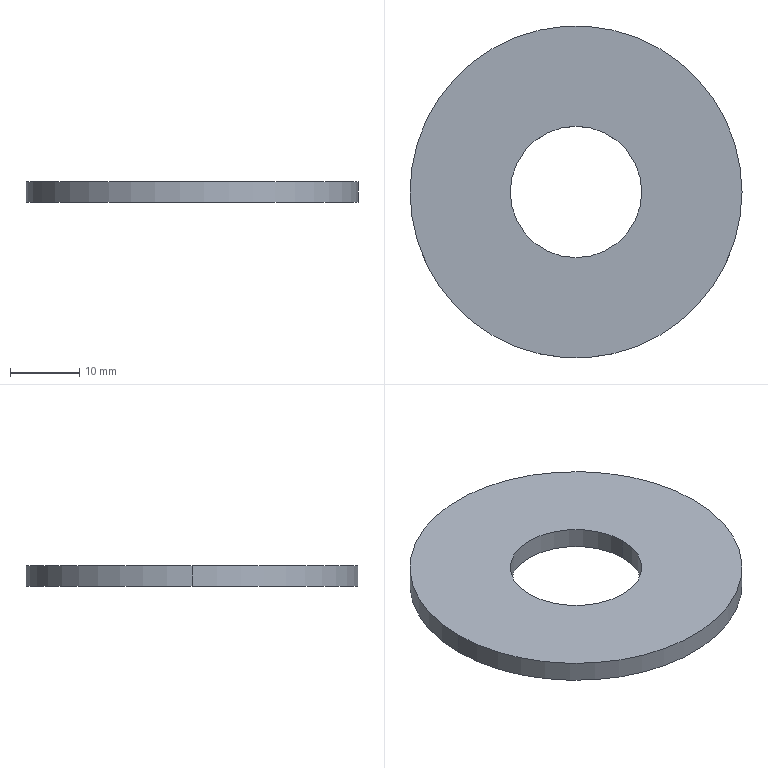Part | SolidWorks | features Extrusion 1 | 1 solid | 6 faces | box 48 x 48 x 3 mm | volume 4578 mm3 | cylinder 4 | plane 2 | commonest cylinder face diameters 19 x2 48 x2
STEP:
#1=CARTESIAN_POINT('',(-9.5,0.,3.));
#2=VERTEX_POINT('',#1);
#3=CARTESIAN_POINT('',(9.5,0.,3.));
#4=VERTEX_POINT('',#3);
#5=CARTESIAN_POINT('',(0.,0.,3.));
#6=DIRECTION('',(0.,0.,1.));
#7=DIRECTION('',(1.,0.,0.));
#8=AXIS2_PLACEMENT_3D('',#5,#6,#7);
#9=CIRCLE('',#8,9.5);
#10=EDGE_CURVE('',#2,#4,#9,.T.);
#11=ORIENTED_EDGE('',*,*,#10,.T.);
#12=CARTESIAN_POINT('',(9.5,0.,0.));
#13=VERTEX_POINT('',#12);
#14=CARTESIAN_POINT('',(9.5,0.,3.));
#15=DIRECTION('',(0.,0.,-1.));
#16=VECTOR('',#15,1000.);
#17=LINE('',#14,#16);
#18=EDGE_CURVE('',#4,#13,#17,.T.);
#19=ORIENTED_EDGE('',*,*,#18,.T.);
#20=CARTESIAN_POINT('',(-9.5,0.,0.));
#21=VERTEX_POINT('',#20);
#22=CARTESIAN_POINT('',(0.,0.,0.));
#23=DIRECTION('',(0.,0.,1.));
#24=DIRECTION('',(1.,0.,0.));
#25=AXIS2_PLACEMENT_3D('',#22,#23,#24);
#26=CIRCLE('',#25,9.5);
#27=EDGE_CURVE('',#21,#13,#26,.T.);
#28=ORIENTED_EDGE('',*,*,#27,.F.);
#29=CARTESIAN_POINT('',(-9.5,0.,3.));
#30=DIRECTION('',(0.,0.,-1.));
#31=VECTOR('',#30,1000.);
#32=LINE('',#29,#31);
#33=EDGE_CURVE('',#2,#21,#32,.T.);
#34=ORIENTED_EDGE('',*,*,#33,.F.);
#35=EDGE_LOOP('',(#11,#19,#28,#34));
#36=FACE_OUTER_BOUND('',#35,.T.);
#37=CARTESIAN_POINT('',(0.,0.,3.));
#38=DIRECTION('',(0.,0.,-1.));
#39=DIRECTION('',(-1.,0.,0.));
#40=AXIS2_PLACEMENT_3D('',#37,#38,#39);
#41=CYLINDRICAL_SURFACE('',#40,9.5);
#42=ADVANCED_FACE('',(#36),#41,.F.);
#43=CARTESIAN_POINT('',(24.,0.,3.));
#44=VERTEX_POINT('',#43);
#45=CARTESIAN_POINT('',(-24.,0.,3.));
#46=VERTEX_POINT('',#45);
#47=CARTESIAN_POINT('',(0.,0.,3.));
#48=DIRECTION('',(0.,0.,1.));
#49=DIRECTION('',(1.,0.,0.));
#50=AXIS2_PLACEMENT_3D('',#47,#48,#49);
#51=CIRCLE('',#50,24.);
#52=EDGE_CURVE('',#44,#46,#51,.T.);
#53=ORIENTED_EDGE('',*,*,#52,.F.);
#54=CARTESIAN_POINT('',(24.,0.,0.));
#55=VERTEX_POINT('',#54);
#56=CARTESIAN_POINT('',(24.,0.,3.));
#57=DIRECTION('',(0.,0.,-1.));
#58=VECTOR('',#57,1000.);
#59=LINE('',#56,#58);
#60=EDGE_CURVE('',#44,#55,#59,.T.);
#61=ORIENTED_EDGE('',*,*,#60,.T.);
#62=CARTESIAN_POINT('',(-24.,0.,0.));
#63=VERTEX_POINT('',#62);
#64=CARTESIAN_POINT('',(0.,0.,0.));
#65=DIRECTION('',(0.,0.,1.));
#66=DIRECTION('',(1.,0.,0.));
#67=AXIS2_PLACEMENT_3D('',#64,#65,#66);
#68=CIRCLE('',#67,24.);
#69=EDGE_CURVE('',#55,#63,#68,.T.);
#70=ORIENTED_EDGE('',*,*,#69,.T.);
#71=CARTESIAN_POINT('',(-24.,0.,3.));
#72=DIRECTION('',(0.,0.,-1.));
#73=VECTOR('',#72,1000.);
#74=LINE('',#71,#73);
#75=EDGE_CURVE('',#46,#63,#74,.T.);
#76=ORIENTED_EDGE('',*,*,#75,.F.);
#77=EDGE_LOOP('',(#53,#61,#70,#76));
#78=FACE_OUTER_BOUND('',#77,.T.);
#79=CARTESIAN_POINT('',(0.,0.,3.));
#80=DIRECTION('',(0.,0.,-1.));
#81=DIRECTION('',(-1.,0.,0.));
#82=AXIS2_PLACEMENT_3D('',#79,#80,#81);
#83=CYLINDRICAL_SURFACE('',#82,24.);
#84=ADVANCED_FACE('',(#78),#83,.T.);
#85=CARTESIAN_POINT('',(0.,0.,3.));
#86=DIRECTION('',(0.,0.,1.));
#87=DIRECTION('',(1.,0.,0.));
#88=AXIS2_PLACEMENT_3D('',#85,#86,#87);
#89=CIRCLE('',#88,24.);
#90=EDGE_CURVE('',#46,#44,#89,.T.);
#91=ORIENTED_EDGE('',*,*,#90,.T.);
#92=ORIENTED_EDGE('',*,*,#52,.T.);
#93=EDGE_LOOP('',(#91,#92));
#94=FACE_OUTER_BOUND('',#93,.T.);
#95=ORIENTED_EDGE('',*,*,#10,.F.);
#96=CARTESIAN_POINT('',(0.,0.,3.));
#97=DIRECTION('',(0.,0.,1.));
#98=DIRECTION('',(1.,0.,0.));
#99=AXIS2_PLACEMENT_3D('',#96,#97,#98);
#100=CIRCLE('',#99,9.5);
#101=EDGE_CURVE('',#4,#2,#100,.T.);
#102=ORIENTED_EDGE('',*,*,#101,.F.);
#103=EDGE_LOOP('',(#95,#102));
#104=FACE_BOUND('',#103,.T.);
#105=CARTESIAN_POINT('',(0.,0.,3.));
#106=DIRECTION('',(0.,0.,1.));
#107=DIRECTION('',(1.,0.,0.));
#108=AXIS2_PLACEMENT_3D('',#105,#106,#107);
#109=PLANE('',#108);
#110=ADVANCED_FACE('',(#94,#104),#109,.T.);
#111=CARTESIAN_POINT('',(0.,0.,0.));
#112=DIRECTION('',(0.,0.,1.));
#113=DIRECTION('',(1.,0.,0.));
#114=AXIS2_PLACEMENT_3D('',#111,#112,#113);
#115=CIRCLE('',#114,24.);
#116=EDGE_CURVE('',#63,#55,#115,.T.);
#117=ORIENTED_EDGE('',*,*,#116,.F.);
#118=ORIENTED_EDGE('',*,*,#69,.F.);
#119=EDGE_LOOP('',(#117,#118));
#120=FACE_OUTER_BOUND('',#119,.T.);
#121=ORIENTED_EDGE('',*,*,#27,.T.);
#122=CARTESIAN_POINT('',(0.,0.,0.));
#123=DIRECTION('',(0.,0.,1.));
#124=DIRECTION('',(1.,0.,0.));
#125=AXIS2_PLACEMENT_3D('',#122,#123,#124);
#126=CIRCLE('',#125,9.5);
#127=EDGE_CURVE('',#13,#21,#126,.T.);
#128=ORIENTED_EDGE('',*,*,#127,.T.);
#129=EDGE_LOOP('',(#121,#128));
#130=FACE_BOUND('',#129,.T.);
#131=CARTESIAN_POINT('',(0.,0.,0.));
#132=DIRECTION('',(0.,0.,1.));
#133=DIRECTION('',(1.,0.,0.));
#134=AXIS2_PLACEMENT_3D('',#131,#132,#133);
#135=PLANE('',#134);
#136=ADVANCED_FACE('',(#120,#130),#135,.F.);
#137=ORIENTED_EDGE('',*,*,#60,.F.);
#138=ORIENTED_EDGE('',*,*,#90,.F.);
#139=ORIENTED_EDGE('',*,*,#75,.T.);
#140=ORIENTED_EDGE('',*,*,#116,.T.);
#141=EDGE_LOOP('',(#137,#138,#139,#140));
#142=FACE_OUTER_BOUND('',#141,.T.);
#143=CARTESIAN_POINT('',(0.,0.,3.));
#144=DIRECTION('',(0.,0.,-1.));
#145=DIRECTION('',(-1.,0.,0.));
#146=AXIS2_PLACEMENT_3D('',#143,#144,#145);
#147=CYLINDRICAL_SURFACE('',#146,24.);
#148=ADVANCED_FACE('',(#142),#147,.T.);
#149=ORIENTED_EDGE('',*,*,#18,.F.);
#150=ORIENTED_EDGE('',*,*,#101,.T.);
#151=ORIENTED_EDGE('',*,*,#33,.T.);
#152=ORIENTED_EDGE('',*,*,#127,.F.);
#153=EDGE_LOOP('',(#149,#150,#151,#152));
#154=FACE_OUTER_BOUND('',#153,.T.);
#155=CARTESIAN_POINT('',(0.,0.,3.));
#156=DIRECTION('',(0.,0.,-1.));
#157=DIRECTION('',(-1.,0.,0.));
#158=AXIS2_PLACEMENT_3D('',#155,#156,#157);
#159=CYLINDRICAL_SURFACE('',#158,9.5);
#160=ADVANCED_FACE('',(#154),#159,.F.);
#161=CLOSED_SHELL('',(#42,#84,#110,#136,#148,#160));
#162=MANIFOLD_SOLID_BREP('',#161);
#163=CARTESIAN_POINT('',(0.,0.,0.));
#164=DIRECTION('',(0.,0.,1.));
#165=DIRECTION('',(1.,0.,0.));
#166=AXIS2_PLACEMENT_3D('',#163,#164,#165);
#167=(LENGTH_UNIT()NAMED_UNIT(*)SI_UNIT(.MILLI.,.METRE.));
#168=UNCERTAINTY_MEASURE_WITH_UNIT(LENGTH_MEASURE(0.00001),#167,'','');
#169=(NAMED_UNIT(*)PLANE_ANGLE_UNIT()SI_UNIT($,.RADIAN.));
#170=(NAMED_UNIT(*)SI_UNIT($,.STERADIAN.)SOLID_ANGLE_UNIT());
#171=(GEOMETRIC_REPRESENTATION_CONTEXT(3)GLOBAL_UNCERTAINTY_ASSIGNED_CONTEXT((#168))GLOBAL_UNIT_ASSIGNED_CONTEXT((#167,#169,#170))REPRESENTATION_CONTEXT('',''));
#172=ADVANCED_BREP_SHAPE_REPRESENTATION('',(#162,#166),#171);